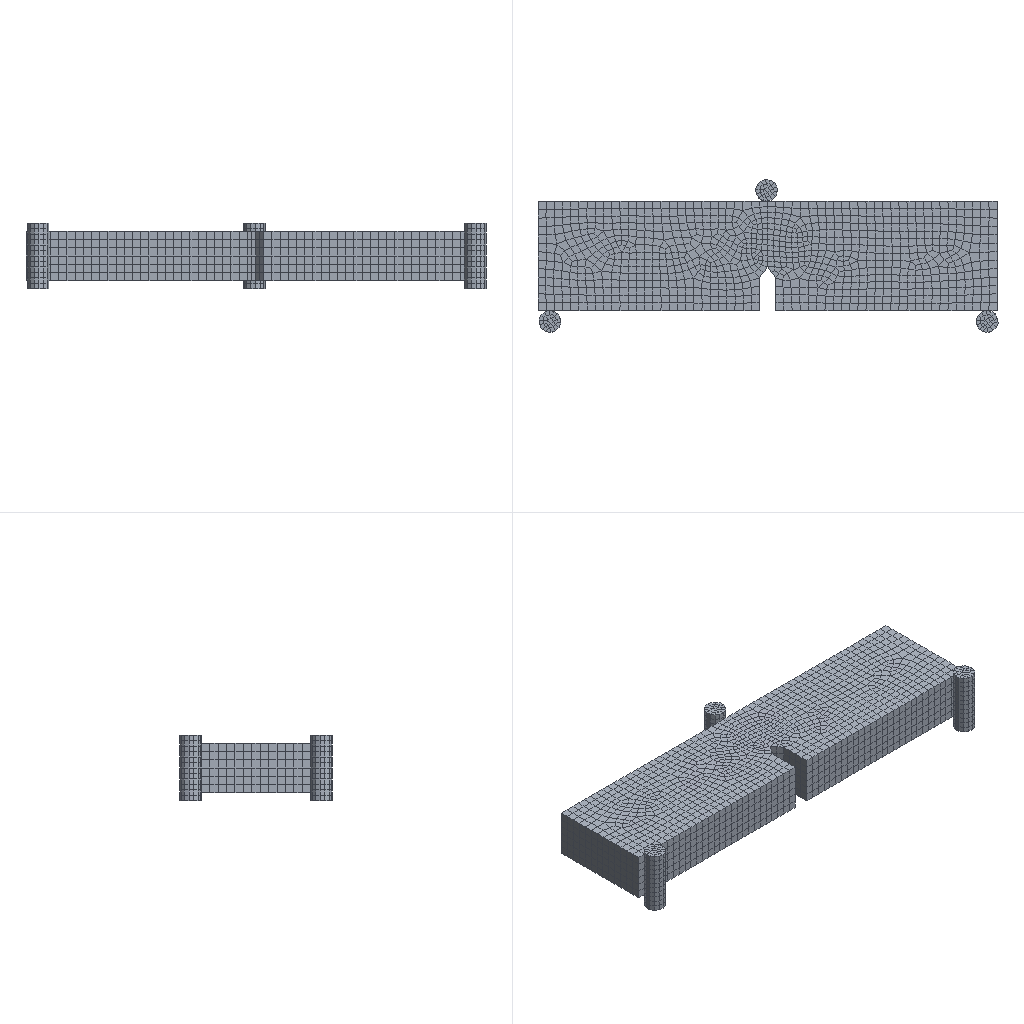Simulation study | abaqus
Set-up summary:
category,name,step,type,value,unit,region
solver,abaqus
solver,version,,,Abaqus/Explicit 2020
units,not stated in the deck,,not stated
analysis,deck,,transient,transient
load_step,Step-1,Step-1,transient,nlgeom=True
contact,interactions,,,general=1 pairs=0 ties=0
load_step,requested,,,1
mesh,nodes,,,8557
mesh,elements,,,6678
element_type,C3D8R,,solid,6606
element_type,COH3D8,,cohesive,72
load,load commands in deck,,count,1
bc,support commands in deck,,count,7
material,COH,,in results
material,MATERIAL-1,,in results
check,setup vs results,,match,"per instance, exact: element labels, types and connectivity; labels of the nodes the elements use; coordinates of those nodes at SINGLE_PRECISION in 4 of 4 instance(s)"
Abaqus input file, long lists of numbers shortened:
*Heading
** Job name: Job-1 Model name: Model-1
** Generated by: Abaqus/CAE 2020
*Preprint, echo=NO, model=NO, history=NO, contact=NO
**
** PARTS
**
*Part, name=ban
*Node
      1,          42.,           0.,           0.
      2,          42.,         -10.,           0.
** (7229 more lines like these left out)
*Element, type=C3D8R
   1, 7144,  394,  385, 7146, 7143, 2861, 2852, 7145
   2,    4,  769,  771,  383,  106, 3236, 3238, 2850
** (5668 more lines like these left out)
*Element, type=COH3D8
5671,   23, 1385,  116,    1, 7144, 7143, 7142, 7141
5672,   23,   24, 1386, 1385, 7144, 7146, 7145, 7143
** (70 more lines like these left out)
*Nset, nset=Set-6, generate
    1,  7231,     1
*Elset, elset=Set-6, generate
    1,  5670,     1
*Elset, elset=CohesiveSeam-1-Elements, generate
 5671,  5742,     1
*Nset, nset=CohesiveSeam-1-TopNodes, generate
 7141,  7231,     1
*Nset, nset=CohesiveSeam-1-BottomNodes
    1,    2,    3,    8,    9,   14,   23,   24,   25,   26,   27,   28,   29,   30,   31,   32
  107,  108,  109,  110,  111,  112,  113,  114,  115,  116,  132,  133,  134,  135,  136,  137
** (4 more lines like these left out)
*Elset, elset=__PickedSurf7_S2, internal, generate
 5671,  5742,     1
*Surface, type=ELEMENT, name=_PickedSurf7, internal
__PickedSurf7_S2, S2
*Elset, elset=_CohesiveSeam-1-TopSurf_S2, internal, generate
 5671,  5742,     1
*Surface, type=ELEMENT, name=CohesiveSeam-1-TopSurf
_CohesiveSeam-1-TopSurf_S2, S2
*Elset, elset=_CohesiveSeam-1-BottomSurf_S1, internal, generate
 5671,  5742,     1
*Surface, type=ELEMENT, name=CohesiveSeam-1-BottomSurf
_CohesiveSeam-1-BottomSurf_S1, S1
** Section: Section-1
*Solid Section, elset=Set-6, material=Material-1
,
** Section: coh
*Cohesive Section, elset=CohesiveSeam-1-Elements, controls=EC-1, material=coh, response=TRACTION SEPARATION
,
*End Part
**
*Part, name=rig
*Node
      1,   1.027,  -1.716,           0.
      2,   1.67,  -1.1,           0.
** (440 more lines like these left out)
*Element, type=C3D8R
  1,  49,  48,  47,  50,  15,  14,  13,  16
  2,  50,  47,  46,  63,  16,  13,  12,  29
** (310 more lines like these left out)
*Nset, nset=Set-1, generate
   1,  442,    1
*Elset, elset=Set-1, generate
   1,  312,    1
** Section: Section-1
*Solid Section, elset=Set-1, material=Material-1
,
*End Part
**
**
** ASSEMBLY
**
*Assembly, name=Assembly
**
*Instance, name=ban-1, part=ban
*End Instance
**
*Instance, name=rig-1, part=rig
   41.819,     1.992,         -1.5
*End Instance
**
*Instance, name=rig-2, part=rig
    2.181,   -21.992,         -1.5
*End Instance
**
*Instance, name=rig-2-lin-2-1, part=rig
   82.181,   -21.992,         -1.5
*End Instance
**
*Node
      1,   41.819,     1.992,          4.5
*Node
      2,   2.181,   -21.992,          4.5
*Node
      3,   82.181,   -21.992,          4.5
*Nset, nset=Set-7
 2, 3
*Nset, nset=Set-8
 1,
*Nset, nset=b_Set-1, instance=rig-1, generate
   1,  442,    1
*Elset, elset=b_Set-1, instance=rig-1, generate
   1,  312,    1
*Nset, nset=b_Set-3, instance=rig-2, generate
   1,  442,    1
*Elset, elset=b_Set-3, instance=rig-2, generate
   1,  312,    1
*Nset, nset=b_Set-5, instance=rig-2-lin-2-1, generate
   1,  442,    1
*Elset, elset=b_Set-5, instance=rig-2-lin-2-1, generate
   1,  312,    1
*Nset, nset=_PickedSet23, internal
 1,
*Nset, nset=_PickedSet25, internal
 2,
*Nset, nset=_PickedSet27, internal
 3,
*Elset, elset=_m_Surf-1_S4, internal, instance=rig-1
   1,   2,   3,  12,  13,  21,  22,  27,  28,  29,  38,  39,  47,  48,  53,  54
  55,  64,  65,  73,  74,  79,  80,  81,  90,  91,  99, 100, 105, 106, 107, 116
** (4 more lines like these left out)
*Elset, elset=_m_Surf-1_S6, internal, instance=rig-1, generate
   4,  290,   26
*Elset, elset=_m_Surf-1_S5, internal, instance=rig-1
  10,  17,  36,  43,  62,  69,  88,  95, 114, 121, 140, 147, 166, 173, 192, 199
 218, 225, 244, 251, 270, 277, 296, 303
*Elset, elset=_m_Surf-1_S3, internal, instance=rig-1
  16,  20,  23,  24,  42,  46,  49,  50,  68,  72,  75,  76,  94,  98, 101, 102
 120, 124, 127, 128, 146, 150, 153, 154, 172, 176, 179, 180, 198, 202, 205, 206
** (1 more lines like these left out)
*Surface, type=ELEMENT, name=m_Surf-1
_m_Surf-1_S4, S4
_m_Surf-1_S6, S6
_m_Surf-1_S5, S5
_m_Surf-1_S3, S3
*Elset, elset=_m_Surf-3_S4, internal, instance=rig-2
   1,   2,   3,  12,  13,  21,  22,  27,  28,  29,  38,  39,  47,  48,  53,  54
  55,  64,  65,  73,  74,  79,  80,  81,  90,  91,  99, 100, 105, 106, 107, 116
** (4 more lines like these left out)
*Elset, elset=_m_Surf-3_S6, internal, instance=rig-2, generate
   4,  290,   26
*Elset, elset=_m_Surf-3_S5, internal, instance=rig-2
  10,  17,  36,  43,  62,  69,  88,  95, 114, 121, 140, 147, 166, 173, 192, 199
 218, 225, 244, 251, 270, 277, 296, 303
*Elset, elset=_m_Surf-3_S3, internal, instance=rig-2
  16,  20,  23,  24,  42,  46,  49,  50,  68,  72,  75,  76,  94,  98, 101, 102
 120, 124, 127, 128, 146, 150, 153, 154, 172, 176, 179, 180, 198, 202, 205, 206
** (1 more lines like these left out)
*Surface, type=ELEMENT, name=m_Surf-3
_m_Surf-3_S4, S4
_m_Surf-3_S6, S6
_m_Surf-3_S5, S5
_m_Surf-3_S3, S3
*Elset, elset=_m_Surf-5_S4, internal, instance=rig-2-lin-2-1
   1,   2,   3,  12,  13,  21,  22,  27,  28,  29,  38,  39,  47,  48,  53,  54
  55,  64,  65,  73,  74,  79,  80,  81,  90,  91,  99, 100, 105, 106, 107, 116
** (4 more lines like these left out)
*Elset, elset=_m_Surf-5_S6, internal, instance=rig-2-lin-2-1, generate
   4,  290,   26
*Elset, elset=_m_Surf-5_S5, internal, instance=rig-2-lin-2-1
  10,  17,  36,  43,  62,  69,  88,  95, 114, 121, 140, 147, 166, 173, 192, 199
 218, 225, 244, 251, 270, 277, 296, 303
*Elset, elset=_m_Surf-5_S3, internal, instance=rig-2-lin-2-1
  16,  20,  23,  24,  42,  46,  49,  50,  68,  72,  75,  76,  94,  98, 101, 102
 120, 124, 127, 128, 146, 150, 153, 154, 172, 176, 179, 180, 198, 202, 205, 206
** (1 more lines like these left out)
*Surface, type=ELEMENT, name=m_Surf-5
_m_Surf-5_S4, S4
_m_Surf-5_S6, S6
_m_Surf-5_S5, S5
_m_Surf-5_S3, S3
*Elset, elset=_s_Surf-1_S5, internal, instance=ban-1
 2886, 2894, 2896, 2897, 2898, 2903, 2906, 2913, 2916, 2990, 2997, 3004, 3009, 3013, 3040, 3351
 3359, 3361, 3362, 3363, 3368, 3371, 3378, 3381, 3455, 3462, 3469, 3474, 3478, 3505, 3816, 3824
** (4 more lines like these left out)
*Elset, elset=_s_Surf-1_S3, internal, instance=ban-1
 2900, 2901, 2904, 2905, 2907, 2908, 2970, 2984, 2991, 2992, 2996, 2998, 3039, 3365, 3366, 3369
 3370, 3372, 3373, 3435, 3449, 3456, 3457, 3461, 3463, 3504, 3830, 3831, 3834, 3835, 3837, 3838
** (3 more lines like these left out)
*Elset, elset=_s_Surf-1_S6, internal, instance=ban-1
    3,   51,   53,   63,   64,   70,   74,  111,  116,  127,  128,  129,  130,  133,  135,  153
  159,  483,  531,  533,  543,  544,  550,  554,  591,  596,  607,  608,  609,  610,  613,  615
** (5 more lines like these left out)
*Elset, elset=_s_Surf-1_S4, internal, instance=ban-1
   32,   39,   40,   57,   62,   71,   72,   73,  102,  139,  160,  512,  519,  520,  537,  542
  551,  552,  553,  582,  619,  640,  992,  999, 1000, 1017, 1022, 1031, 1032, 1033, 1062, 1099
** (3 more lines like these left out)
*Surface, type=ELEMENT, name=s_Surf-1
_s_Surf-1_S5, S5
_s_Surf-1_S3, S3
_s_Surf-1_S6, S6
_s_Surf-1_S4, S4
*Elset, elset=_s_Surf-3_S5, internal, instance=ban-1
   15,   17,   19,   20,   21,   27,   30,   91,  118,  122,  123,  131,  134,  137,  156,  495
  497,  499,  500,  501,  507,  510,  571,  598,  602,  603,  611,  614,  617,  636,  975,  977
** (4 more lines like these left out)
*Elset, elset=_s_Surf-3_S3, internal, instance=ban-1
   23,   24,   25,   28,   29,   31,   37,   97,  104,  115,  121,  124,  503,  504,  505,  508
  509,  511,  517,  577,  584,  595,  601,  604,  983,  984,  985,  988,  989,  991,  997, 1057
** (3 more lines like these left out)
*Surface, type=ELEMENT, name=s_Surf-3
_s_Surf-3_S5, S5
_s_Surf-3_S3, S3
*Elset, elset=_s_Surf-5_S6, internal, instance=ban-1
 2884, 2910, 2927, 2928, 2938, 2939, 2940, 2942, 2946, 2950, 3001, 3002, 3003, 3005, 3010, 3034
 3349, 3375, 3392, 3393, 3403, 3404, 3405, 3407, 3411, 3415, 3466, 3467, 3468, 3470, 3475, 3499
** (4 more lines like these left out)
*Elset, elset=_s_Surf-5_S4, internal, instance=ban-1
 2917, 2918, 2931, 2932, 2947, 2948, 2949, 2977, 3011, 3016, 3020, 3382, 3383, 3396, 3397, 3412
 3413, 3414, 3442, 3476, 3481, 3485, 3847, 3848, 3861, 3862, 3877, 3878, 3879, 3907, 3941, 3946
** (3 more lines like these left out)
*Surface, type=ELEMENT, name=s_Surf-5
_s_Surf-5_S6, S6
_s_Surf-5_S4, S4
** Constraint: Constraint-1
*Rigid Body, ref node=_PickedSet23, elset=b_Set-1
** Constraint: Constraint-2
*Rigid Body, ref node=_PickedSet25, elset=b_Set-3
** Constraint: Constraint-3
*Rigid Body, ref node=_PickedSet27, elset=b_Set-5
*End Assembly
**
** ELEMENT CONTROLS
**
*Section Controls, name=EC-1, ELEMENT DELETION=YES
1., 1., 1.
*Amplitude, name=Amp-1
             0.,              0.,             0.1,              1.
**
** MATERIALS
**
*Material, name=Material-1
*Density
 8e-09,
*Elastic
250000., 0.33
*Plastic
350.,0.
*Material, name=coh
*Damage Initiation, criterion=MAXS
250.,250.,250.
*Damage Evolution, type=DISPLACEMENT
 1e-11,
*Density
 8e-09,
*Elastic, type=TRACTION
150000.,150000.,150000.
**
** INTERACTION PROPERTIES
**
*Surface Interaction, name=IntProp-1
*Friction
 0.2,
*Surface Behavior, pressure-overclosure=HARD
** ----------------------------------------------------------------
**
** STEP: Step-1
**
*Step, name=Step-1, nlgeom=YES
*Dynamic, Explicit
, 0.1
*Bulk Viscosity
0.06, 1.2
**
** BOUNDARY CONDITIONS
**
** Name: BC-1 Type: 对称/反对称/完全固定
*Boundary
Set-7, ENCASTRE
** Name: [REDACTED] : Displacement/rotation angle
*Boundary, amplitude=Amp-1
Set-8, 1, 1
Set-8, 2, 2, -1.
Set-8, 3, 3
Set-8, 4, 4
Set-8, 5, 5
Set-8, 6, 6
**
** INTERACTIONS
**
** Interaction: Int-4
*Contact, op=NEW
*Contact Inclusions, ALL EXTERIOR
*Contact Property Assignment
 ,  , IntProp-1
**
** OUTPUT REQUESTS
**
*Restart, write, number interval=1, time marks=NO
**
** FIELD OUTPUT: F-Output-1
**
*Output, field, number interval=50
*Node Output
A, CF, RF, RM, U, V
*Element Output, directions=YES
E, EVF, LE, MISES, MISESMAX, MISESONLY, PE, PEEQ, PEEQMAX, PEEQT, PEEQVAVG, PEMAG, PEVAVG, PRESSONLY, S, SDEG
SF, STATUS, SVAVG, YIELDPOT
*Contact Output
CDISP, CSTRESS
**
** HISTORY OUTPUT: H-Output-1
**
*Output, history, time interval=2e-06
*Node Output, nset=Set-8
RF2, U2
*End Step
Results summary:
result,step,Step-1,completed,increments=899301 time=0.1/0.1
result,analysis,,,transient
result,last_loadstep,,,1
result,analysis steps,,count,1
result,primary field,,,U
result,reaction total,,FX,0.421,model units
result,reaction total,,FY,2.176,model units
result,reaction total,,FZ,-0.2049,model units